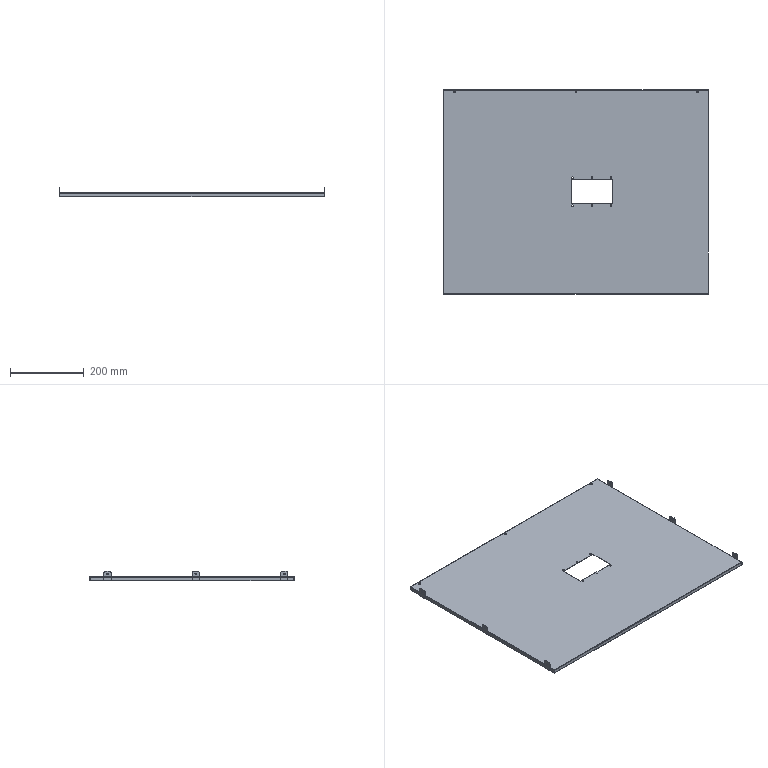Part | STEP file | RJWD-DY-0109_-0001 | 10 solids | 149 faces | box 722 x 555.2 x 25 mm | volume 417115 mm3 | plane 79 | cylinder 64 | spline 6 | commonest cylinder face diameters 4 x24 5 x12 10 x12 7.9 x6 0.4 x5 2.4 x5